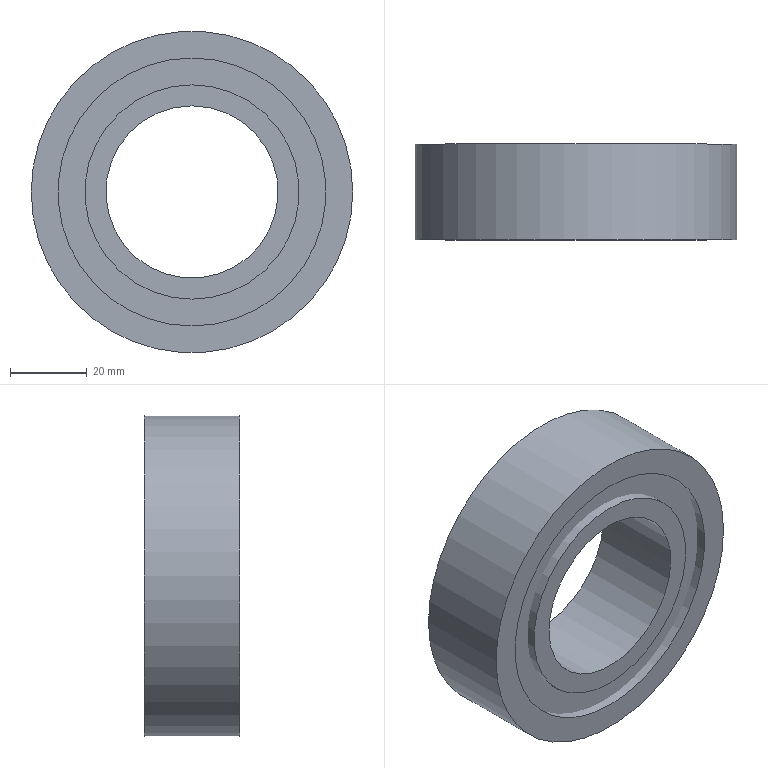Part | NX | features DATUM_CSYS 4, EXTRUDE 3, SKETCH 3 | 3 solids | 12 faces | box 84 x 25 x 84 mm | volume 95815 mm3 | plane 6 | cylinder 6 | commonest cylinder face diameters 45 x1 55 x1 56 x1 70 x1 71 x1 84 x1
STEP:
#1=CARTESIAN_POINT('',(0.,-2.5,-27.5));
#2=VERTEX_POINT('',#1);
#3=CARTESIAN_POINT('',(0.,-2.5,0.));
#4=DIRECTION('',(0.,-1.,0.));
#5=DIRECTION('',(0.,0.,-1.));
#6=AXIS2_PLACEMENT_3D('',#3,#4,#5);
#7=CIRCLE('',#6,27.5);
#8=EDGE_CURVE('',#2,#2,#7,.T.);
#9=ORIENTED_EDGE('',*,*,#8,.T.);
#10=EDGE_LOOP('',(#9));
#11=FACE_BOUND('',#10,.T.);
#12=CARTESIAN_POINT('',(0.,-2.5,-35.5));
#13=VERTEX_POINT('',#12);
#14=CARTESIAN_POINT('',(0.,-2.5,0.));
#15=DIRECTION('',(0.,-1.,0.));
#16=DIRECTION('',(0.,0.,-1.));
#17=AXIS2_PLACEMENT_3D('',#14,#15,#16);
#18=CIRCLE('',#17,35.5);
#19=EDGE_CURVE('',#13,#13,#18,.T.);
#20=ORIENTED_EDGE('',*,*,#19,.F.);
#21=EDGE_LOOP('',(#20));
#22=FACE_BOUND('',#21,.T.);
#23=CARTESIAN_POINT('',(0.,-2.5,0.));
#24=DIRECTION('',(0.,-1.,0.));
#25=DIRECTION('',(0.,0.,-1.));
#26=AXIS2_PLACEMENT_3D('',#23,#24,#25);
#27=PLANE('',#26);
#28=ADVANCED_FACE('',(#11,#22),#27,.F.);
#29=CARTESIAN_POINT('',(0.,-22.5,-27.5));
#30=VERTEX_POINT('',#29);
#31=CARTESIAN_POINT('',(0.,-22.5,0.));
#32=DIRECTION('',(0.,-1.,0.));
#33=DIRECTION('',(0.,0.,-1.));
#34=AXIS2_PLACEMENT_3D('',#31,#32,#33);
#35=CIRCLE('',#34,27.5);
#36=EDGE_CURVE('',#30,#30,#35,.T.);
#37=ORIENTED_EDGE('',*,*,#36,.F.);
#38=EDGE_LOOP('',(#37));
#39=FACE_BOUND('',#38,.T.);
#40=CARTESIAN_POINT('',(0.,-22.5,-35.5));
#41=VERTEX_POINT('',#40);
#42=CARTESIAN_POINT('',(0.,-22.5,0.));
#43=DIRECTION('',(0.,-1.,0.));
#44=DIRECTION('',(0.,0.,-1.));
#45=AXIS2_PLACEMENT_3D('',#42,#43,#44);
#46=CIRCLE('',#45,35.5);
#47=EDGE_CURVE('',#41,#41,#46,.T.);
#48=ORIENTED_EDGE('',*,*,#47,.T.);
#49=EDGE_LOOP('',(#48));
#50=FACE_BOUND('',#49,.T.);
#51=CARTESIAN_POINT('',(0.,-22.5,0.));
#52=DIRECTION('',(0.,-1.,0.));
#53=DIRECTION('',(0.,0.,-1.));
#54=AXIS2_PLACEMENT_3D('',#51,#52,#53);
#55=PLANE('',#54);
#56=ADVANCED_FACE('',(#39,#50),#55,.T.);
#57=ORIENTED_EDGE('',*,*,#8,.F.);
#58=EDGE_LOOP('',(#57));
#59=FACE_BOUND('',#58,.T.);
#60=ORIENTED_EDGE('',*,*,#36,.T.);
#61=EDGE_LOOP('',(#60));
#62=FACE_BOUND('',#61,.T.);
#63=CARTESIAN_POINT('',(0.,-2.5,0.));
#64=DIRECTION('',(0.,-1.,0.));
#65=DIRECTION('',(0.,0.,-1.));
#66=AXIS2_PLACEMENT_3D('',#63,#64,#65);
#67=CYLINDRICAL_SURFACE('',#66,27.5);
#68=ADVANCED_FACE('',(#59,#62),#67,.F.);
#69=ORIENTED_EDGE('',*,*,#19,.T.);
#70=EDGE_LOOP('',(#69));
#71=FACE_BOUND('',#70,.T.);
#72=ORIENTED_EDGE('',*,*,#47,.F.);
#73=EDGE_LOOP('',(#72));
#74=FACE_BOUND('',#73,.T.);
#75=CARTESIAN_POINT('',(0.,-2.5,0.));
#76=DIRECTION('',(0.,-1.,0.));
#77=DIRECTION('',(0.,0.,-1.));
#78=AXIS2_PLACEMENT_3D('',#75,#76,#77);
#79=CYLINDRICAL_SURFACE('',#78,35.5);
#80=ADVANCED_FACE('',(#71,#74),#79,.T.);
#81=CLOSED_SHELL('',(#28,#56,#68,#80));
#82=MANIFOLD_SOLID_BREP('',#81);
#83=CARTESIAN_POINT('',(0.,-25.,28.));
#84=VERTEX_POINT('',#83);
#85=CARTESIAN_POINT('',(0.,-25.,0.));
#86=DIRECTION('',(0.,1.,0.));
#87=DIRECTION('',(0.,0.,1.));
#88=AXIS2_PLACEMENT_3D('',#85,#86,#87);
#89=CIRCLE('',#88,28.);
#90=EDGE_CURVE('',#84,#84,#89,.T.);
#91=ORIENTED_EDGE('',*,*,#90,.F.);
#92=EDGE_LOOP('',(#91));
#93=FACE_BOUND('',#92,.T.);
#94=CARTESIAN_POINT('',(0.,-25.,22.5));
#95=VERTEX_POINT('',#94);
#96=CARTESIAN_POINT('',(0.,-25.,0.));
#97=DIRECTION('',(0.,1.,0.));
#98=DIRECTION('',(0.,0.,1.));
#99=AXIS2_PLACEMENT_3D('',#96,#97,#98);
#100=CIRCLE('',#99,22.5);
#101=EDGE_CURVE('',#95,#95,#100,.T.);
#102=ORIENTED_EDGE('',*,*,#101,.T.);
#103=EDGE_LOOP('',(#102));
#104=FACE_BOUND('',#103,.T.);
#105=CARTESIAN_POINT('',(0.,-25.,0.));
#106=DIRECTION('',(0.,1.,0.));
#107=DIRECTION('',(0.,0.,1.));
#108=AXIS2_PLACEMENT_3D('',#105,#106,#107);
#109=PLANE('',#108);
#110=ADVANCED_FACE('',(#93,#104),#109,.F.);
#111=CARTESIAN_POINT('',(0.,0.,28.));
#112=VERTEX_POINT('',#111);
#113=CARTESIAN_POINT('',(0.,0.,0.));
#114=DIRECTION('',(0.,1.,0.));
#115=DIRECTION('',(0.,0.,1.));
#116=AXIS2_PLACEMENT_3D('',#113,#114,#115);
#117=CIRCLE('',#116,28.);
#118=EDGE_CURVE('',#112,#112,#117,.T.);
#119=ORIENTED_EDGE('',*,*,#118,.T.);
#120=EDGE_LOOP('',(#119));
#121=FACE_BOUND('',#120,.T.);
#122=CARTESIAN_POINT('',(0.,0.,22.5));
#123=VERTEX_POINT('',#122);
#124=CARTESIAN_POINT('',(0.,0.,0.));
#125=DIRECTION('',(0.,1.,0.));
#126=DIRECTION('',(0.,0.,1.));
#127=AXIS2_PLACEMENT_3D('',#124,#125,#126);
#128=CIRCLE('',#127,22.5);
#129=EDGE_CURVE('',#123,#123,#128,.T.);
#130=ORIENTED_EDGE('',*,*,#129,.F.);
#131=EDGE_LOOP('',(#130));
#132=FACE_BOUND('',#131,.T.);
#133=CARTESIAN_POINT('',(0.,0.,0.));
#134=DIRECTION('',(0.,1.,0.));
#135=DIRECTION('',(0.,0.,1.));
#136=AXIS2_PLACEMENT_3D('',#133,#134,#135);
#137=PLANE('',#136);
#138=ADVANCED_FACE('',(#121,#132),#137,.T.);
#139=ORIENTED_EDGE('',*,*,#90,.T.);
#140=EDGE_LOOP('',(#139));
#141=FACE_BOUND('',#140,.T.);
#142=ORIENTED_EDGE('',*,*,#118,.F.);
#143=EDGE_LOOP('',(#142));
#144=FACE_BOUND('',#143,.T.);
#145=CARTESIAN_POINT('',(0.,-25.,0.));
#146=DIRECTION('',(0.,1.,0.));
#147=DIRECTION('',(0.,0.,1.));
#148=AXIS2_PLACEMENT_3D('',#145,#146,#147);
#149=CYLINDRICAL_SURFACE('',#148,28.);
#150=ADVANCED_FACE('',(#141,#144),#149,.T.);
#151=ORIENTED_EDGE('',*,*,#101,.F.);
#152=EDGE_LOOP('',(#151));
#153=FACE_BOUND('',#152,.T.);
#154=ORIENTED_EDGE('',*,*,#129,.T.);
#155=EDGE_LOOP('',(#154));
#156=FACE_BOUND('',#155,.T.);
#157=CARTESIAN_POINT('',(0.,-25.,0.));
#158=DIRECTION('',(0.,1.,0.));
#159=DIRECTION('',(0.,0.,1.));
#160=AXIS2_PLACEMENT_3D('',#157,#158,#159);
#161=CYLINDRICAL_SURFACE('',#160,22.5);
#162=ADVANCED_FACE('',(#153,#156),#161,.F.);
#163=CLOSED_SHELL('',(#110,#138,#150,#162));
#164=MANIFOLD_SOLID_BREP('',#163);
#165=CARTESIAN_POINT('',(0.,-25.,35.));
#166=VERTEX_POINT('',#165);
#167=CARTESIAN_POINT('',(0.,-25.,0.));
#168=DIRECTION('',(0.,1.,0.));
#169=DIRECTION('',(0.,0.,1.));
#170=AXIS2_PLACEMENT_3D('',#167,#168,#169);
#171=CIRCLE('',#170,35.);
#172=EDGE_CURVE('',#166,#166,#171,.F.);
#173=ORIENTED_EDGE('',*,*,#172,.F.);
#174=EDGE_LOOP('',(#173));
#175=FACE_BOUND('',#174,.T.);
#176=CARTESIAN_POINT('',(42.,-25.,0.));
#177=VERTEX_POINT('',#176);
#178=CARTESIAN_POINT('',(0.,-25.,0.));
#179=DIRECTION('',(0.,-1.,0.));
#180=DIRECTION('',(1.,0.,0.));
#181=AXIS2_PLACEMENT_3D('',#178,#179,#180);
#182=CIRCLE('',#181,42.);
#183=EDGE_CURVE('',#177,#177,#182,.T.);
#184=ORIENTED_EDGE('',*,*,#183,.T.);
#185=EDGE_LOOP('',(#184));
#186=FACE_BOUND('',#185,.T.);
#187=CARTESIAN_POINT('',(0.,-25.,0.));
#188=DIRECTION('',(0.,1.,0.));
#189=DIRECTION('',(0.,0.,1.));
#190=AXIS2_PLACEMENT_3D('',#187,#188,#189);
#191=PLANE('',#190);
#192=ADVANCED_FACE('',(#175,#186),#191,.F.);
#193=CARTESIAN_POINT('',(0.,0.,35.));
#194=VERTEX_POINT('',#193);
#195=CARTESIAN_POINT('',(0.,0.,0.));
#196=DIRECTION('',(0.,1.,0.));
#197=DIRECTION('',(0.,0.,1.));
#198=AXIS2_PLACEMENT_3D('',#195,#196,#197);
#199=CIRCLE('',#198,35.);
#200=EDGE_CURVE('',#194,#194,#199,.F.);
#201=ORIENTED_EDGE('',*,*,#200,.T.);
#202=EDGE_LOOP('',(#201));
#203=FACE_BOUND('',#202,.T.);
#204=CARTESIAN_POINT('',(42.,0.,0.));
#205=VERTEX_POINT('',#204);
#206=CARTESIAN_POINT('',(0.,0.,0.));
#207=DIRECTION('',(0.,-1.,0.));
#208=DIRECTION('',(1.,0.,0.));
#209=AXIS2_PLACEMENT_3D('',#206,#207,#208);
#210=CIRCLE('',#209,42.);
#211=EDGE_CURVE('',#205,#205,#210,.T.);
#212=ORIENTED_EDGE('',*,*,#211,.F.);
#213=EDGE_LOOP('',(#212));
#214=FACE_BOUND('',#213,.T.);
#215=CARTESIAN_POINT('',(0.,0.,0.));
#216=DIRECTION('',(0.,1.,0.));
#217=DIRECTION('',(0.,0.,1.));
#218=AXIS2_PLACEMENT_3D('',#215,#216,#217);
#219=PLANE('',#218);
#220=ADVANCED_FACE('',(#203,#214),#219,.T.);
#221=ORIENTED_EDGE('',*,*,#172,.T.);
#222=EDGE_LOOP('',(#221));
#223=FACE_BOUND('',#222,.T.);
#224=ORIENTED_EDGE('',*,*,#200,.F.);
#225=EDGE_LOOP('',(#224));
#226=FACE_BOUND('',#225,.T.);
#227=CARTESIAN_POINT('',(0.,-25.,0.));
#228=DIRECTION('',(0.,1.,0.));
#229=DIRECTION('',(0.,0.,1.));
#230=AXIS2_PLACEMENT_3D('',#227,#228,#229);
#231=CYLINDRICAL_SURFACE('',#230,35.);
#232=ADVANCED_FACE('',(#223,#226),#231,.F.);
#233=ORIENTED_EDGE('',*,*,#183,.F.);
#234=EDGE_LOOP('',(#233));
#235=FACE_BOUND('',#234,.T.);
#236=ORIENTED_EDGE('',*,*,#211,.T.);
#237=EDGE_LOOP('',(#236));
#238=FACE_BOUND('',#237,.T.);
#239=CARTESIAN_POINT('',(0.,-25.,0.));
#240=DIRECTION('',(0.,1.,0.));
#241=DIRECTION('',(0.,0.,1.));
#242=AXIS2_PLACEMENT_3D('',#239,#240,#241);
#243=CYLINDRICAL_SURFACE('',#242,42.);
#244=ADVANCED_FACE('',(#235,#238),#243,.T.);
#245=CLOSED_SHELL('',(#192,#220,#232,#244));
#246=MANIFOLD_SOLID_BREP('',#245);
#247=(LENGTH_UNIT()NAMED_UNIT(*)SI_UNIT(.MILLI.,.METRE.));
#248=UNCERTAINTY_MEASURE_WITH_UNIT(LENGTH_MEASURE(0.00001),#247,'','');
#249=(NAMED_UNIT(*)PLANE_ANGLE_UNIT()SI_UNIT($,.RADIAN.));
#250=(NAMED_UNIT(*)SI_UNIT($,.STERADIAN.)SOLID_ANGLE_UNIT());
#251=(GEOMETRIC_REPRESENTATION_CONTEXT(3)GLOBAL_UNCERTAINTY_ASSIGNED_CONTEXT((#248))GLOBAL_UNIT_ASSIGNED_CONTEXT((#247,#249,#250))REPRESENTATION_CONTEXT('',''));
#252=ADVANCED_BREP_SHAPE_REPRESENTATION('',(#82,#164,#246),#251);